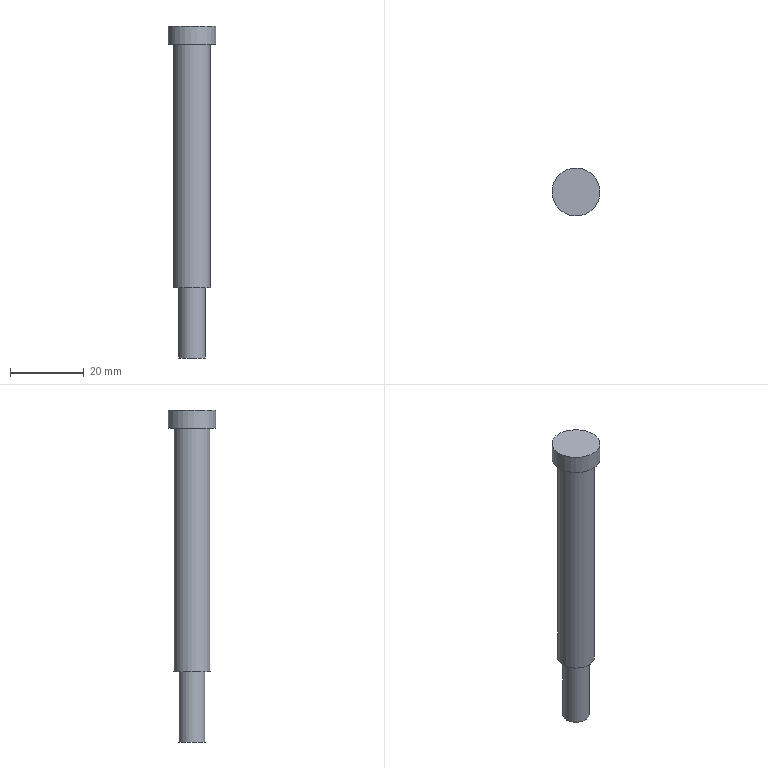Part | NX | features solid 2 | 1 solid | 7 faces | box 13 x 13 x 90 mm | volume 6600 mm3 | plane 4 | cylinder 3 | commonest cylinder face diameters 7.1 x1 10 x1 13 x1
STEP:
#1=CARTESIAN_POINT('',(221.151,-100.003,8.));
#2=VERTEX_POINT('',#1);
#3=CARTESIAN_POINT('',(216.151,-100.003,8.));
#4=DIRECTION('',(0.,0.,1.));
#5=DIRECTION('',(1.,0.,0.));
#6=AXIS2_PLACEMENT_3D('',#3,#4,#5);
#7=CIRCLE('',#6,5.);
#8=EDGE_CURVE('',#2,#2,#7,.T.);
#9=ORIENTED_EDGE('',*,*,#8,.T.);
#10=EDGE_LOOP('',(#9));
#11=FACE_BOUND('',#10,.T.);
#12=CARTESIAN_POINT('',(221.151,-100.003,74.));
#13=VERTEX_POINT('',#12);
#14=CARTESIAN_POINT('',(216.151,-100.003,74.));
#15=DIRECTION('',(0.,0.,1.));
#16=DIRECTION('',(1.,0.,0.));
#17=AXIS2_PLACEMENT_3D('',#14,#15,#16);
#18=CIRCLE('',#17,5.);
#19=EDGE_CURVE('',#13,#13,#18,.T.);
#20=ORIENTED_EDGE('',*,*,#19,.F.);
#21=EDGE_LOOP('',(#20));
#22=FACE_BOUND('',#21,.T.);
#23=CARTESIAN_POINT('',(216.151,-100.003,79.));
#24=DIRECTION('',(0.,0.,-1.));
#25=DIRECTION('',(-1.,0.,0.));
#26=AXIS2_PLACEMENT_3D('',#23,#24,#25);
#27=CYLINDRICAL_SURFACE('',#26,5.);
#28=ADVANCED_FACE('',(#11,#22),#27,.T.);
#29=CARTESIAN_POINT('',(219.701,-100.003,8.));
#30=VERTEX_POINT('',#29);
#31=CARTESIAN_POINT('',(216.151,-100.003,8.));
#32=DIRECTION('',(0.,0.,1.));
#33=DIRECTION('',(1.,0.,0.));
#34=AXIS2_PLACEMENT_3D('',#31,#32,#33);
#35=CIRCLE('',#34,3.55);
#36=EDGE_CURVE('',#30,#30,#35,.T.);
#37=ORIENTED_EDGE('',*,*,#36,.T.);
#38=EDGE_LOOP('',(#37));
#39=FACE_BOUND('',#38,.T.);
#40=ORIENTED_EDGE('',*,*,#8,.F.);
#41=EDGE_LOOP('',(#40));
#42=FACE_BOUND('',#41,.T.);
#43=CARTESIAN_POINT('',(216.151,-100.003,8.));
#44=DIRECTION('',(0.,0.,1.));
#45=DIRECTION('',(1.,0.,0.));
#46=AXIS2_PLACEMENT_3D('',#43,#44,#45);
#47=PLANE('',#46);
#48=ADVANCED_FACE('',(#39,#42),#47,.F.);
#49=CARTESIAN_POINT('',(219.701,-100.003,-11.));
#50=VERTEX_POINT('',#49);
#51=CARTESIAN_POINT('',(216.151,-100.003,-11.));
#52=DIRECTION('',(0.,0.,1.));
#53=DIRECTION('',(1.,0.,0.));
#54=AXIS2_PLACEMENT_3D('',#51,#52,#53);
#55=CIRCLE('',#54,3.55);
#56=EDGE_CURVE('',#50,#50,#55,.T.);
#57=ORIENTED_EDGE('',*,*,#56,.T.);
#58=EDGE_LOOP('',(#57));
#59=FACE_BOUND('',#58,.T.);
#60=ORIENTED_EDGE('',*,*,#36,.F.);
#61=EDGE_LOOP('',(#60));
#62=FACE_BOUND('',#61,.T.);
#63=CARTESIAN_POINT('',(216.151,-100.003,-11.));
#64=DIRECTION('',(0.,0.,1.));
#65=DIRECTION('',(1.,0.,0.));
#66=AXIS2_PLACEMENT_3D('',#63,#64,#65);
#67=CYLINDRICAL_SURFACE('',#66,3.55);
#68=ADVANCED_FACE('',(#59,#62),#67,.T.);
#69=ORIENTED_EDGE('',*,*,#56,.F.);
#70=EDGE_LOOP('',(#69));
#71=FACE_BOUND('',#70,.T.);
#72=CARTESIAN_POINT('',(216.151,-100.003,-11.));
#73=DIRECTION('',(0.,0.,1.));
#74=DIRECTION('',(1.,0.,0.));
#75=AXIS2_PLACEMENT_3D('',#72,#73,#74);
#76=PLANE('',#75);
#77=ADVANCED_FACE('',(#71),#76,.F.);
#78=CARTESIAN_POINT('',(212.901,-105.632,74.));
#79=VERTEX_POINT('',#78);
#80=CARTESIAN_POINT('',(216.151,-100.003,74.));
#81=DIRECTION('',(0.,0.,1.));
#82=DIRECTION('',(-0.5,-0.866,0.));
#83=AXIS2_PLACEMENT_3D('',#80,#81,#82);
#84=CIRCLE('',#83,6.5);
#85=EDGE_CURVE('',#79,#79,#84,.T.);
#86=ORIENTED_EDGE('',*,*,#85,.F.);
#87=EDGE_LOOP('',(#86));
#88=FACE_BOUND('',#87,.T.);
#89=ORIENTED_EDGE('',*,*,#19,.T.);
#90=EDGE_LOOP('',(#89));
#91=FACE_BOUND('',#90,.T.);
#92=CARTESIAN_POINT('',(216.151,-100.003,74.));
#93=DIRECTION('',(0.,0.,1.));
#94=DIRECTION('',(-0.5,-0.866,0.));
#95=AXIS2_PLACEMENT_3D('',#92,#93,#94);
#96=PLANE('',#95);
#97=ADVANCED_FACE('',(#88,#91),#96,.F.);
#98=ORIENTED_EDGE('',*,*,#85,.T.);
#99=EDGE_LOOP('',(#98));
#100=FACE_BOUND('',#99,.T.);
#101=CARTESIAN_POINT('',(212.901,-105.632,79.));
#102=VERTEX_POINT('',#101);
#103=CARTESIAN_POINT('',(216.151,-100.003,79.));
#104=DIRECTION('',(0.,0.,1.));
#105=DIRECTION('',(-0.5,-0.866,0.));
#106=AXIS2_PLACEMENT_3D('',#103,#104,#105);
#107=CIRCLE('',#106,6.5);
#108=EDGE_CURVE('',#102,#102,#107,.T.);
#109=ORIENTED_EDGE('',*,*,#108,.F.);
#110=EDGE_LOOP('',(#109));
#111=FACE_BOUND('',#110,.T.);
#112=CARTESIAN_POINT('',(216.151,-100.003,74.));
#113=DIRECTION('',(0.,0.,1.));
#114=DIRECTION('',(-0.5,-0.866,0.));
#115=AXIS2_PLACEMENT_3D('',#112,#113,#114);
#116=CYLINDRICAL_SURFACE('',#115,6.5);
#117=ADVANCED_FACE('',(#100,#111),#116,.T.);
#118=ORIENTED_EDGE('',*,*,#108,.T.);
#119=EDGE_LOOP('',(#118));
#120=FACE_BOUND('',#119,.T.);
#121=CARTESIAN_POINT('',(216.151,-100.003,79.));
#122=DIRECTION('',(0.,0.,1.));
#123=DIRECTION('',(1.,0.,0.));
#124=AXIS2_PLACEMENT_3D('',#121,#122,#123);
#125=PLANE('',#124);
#126=ADVANCED_FACE('',(#120),#125,.T.);
#127=CLOSED_SHELL('',(#28,#48,#68,#77,#97,#117,#126));
#128=MANIFOLD_SOLID_BREP('',#127);
#129=(LENGTH_UNIT()NAMED_UNIT(*)SI_UNIT(.MILLI.,.METRE.));
#130=UNCERTAINTY_MEASURE_WITH_UNIT(LENGTH_MEASURE(0.00001),#129,'','');
#131=(NAMED_UNIT(*)PLANE_ANGLE_UNIT()SI_UNIT($,.RADIAN.));
#132=(NAMED_UNIT(*)SI_UNIT($,.STERADIAN.)SOLID_ANGLE_UNIT());
#133=(GEOMETRIC_REPRESENTATION_CONTEXT(3)GLOBAL_UNCERTAINTY_ASSIGNED_CONTEXT((#130))GLOBAL_UNIT_ASSIGNED_CONTEXT((#129,#131,#132))REPRESENTATION_CONTEXT('',''));
#134=ADVANCED_BREP_SHAPE_REPRESENTATION('',(#128),#133);